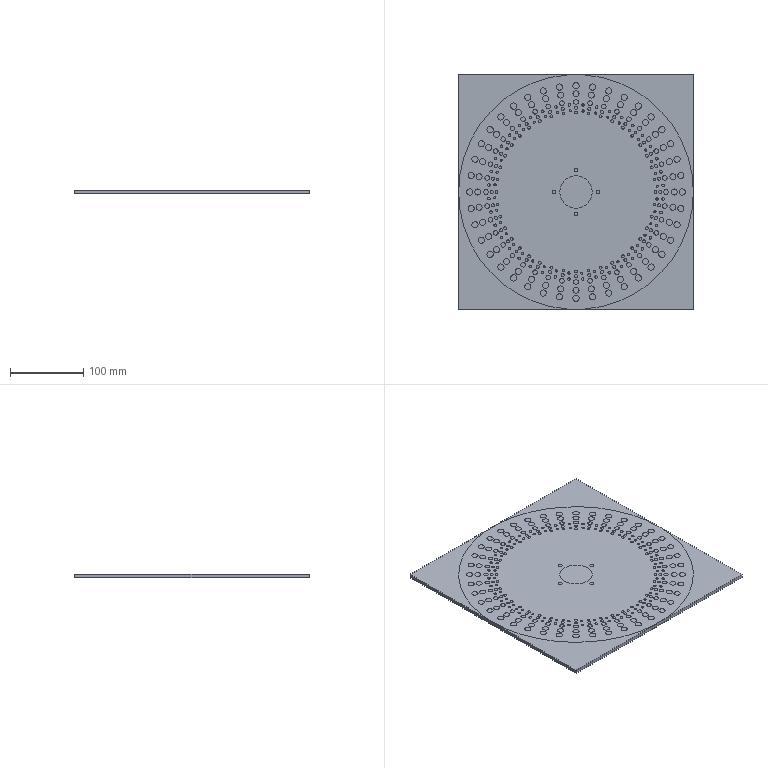NC program | NX | posted with a generic post | part box 320 x 320 x 5 mm
Lines 42718 to 43626 of 63198:
(等高外形_COPY , TOOL : D17R0.8圆鼻飞刀)
N85416 T07 M6
N85418 /M1
N85420 G54
N85422 G17 G0 G90 X-7.068 Y-3.296 S2000 M3
N85424 G43 Z20. H7
N85426 Z0.4
N85428 G94 G1 Z0.2 F1600.
N85430 G3 X-4.906 Y-7.025 R5.1
N85432 X-4.287 Y-7.416 R8.144 F2000.
N85434 X-2.341 Y-8.24 R8.441
N85436 X2.351 Y-8.239 R8.565
N85438 G1 X2.889 Y-8.056
N85440 G3 X4.942 Y-6.996 R7.82
N85442 G1 X5.476 Y-6.59
N85444 X5.768 Y-6.334
N85446 G3 X7.415 Y-4.289 R8.348
N85448 X8.239 Y-2.349 R8.176
N85450 X8.242 Y2.35 R8.507
N85452 G1 X8.238 Y2.355
N85454 G3 X7.418 Y4.288 R8.355
N85456 G1 X7.415 Y4.291
N85458 G3 X5.772 Y6.333 R8.386
N85460 G1 X5.514 Y6.562
N85462 X5.476 Y6.591
N85464 X4.943 Y6.999
N85466 G3 X2.356 Y8.238 R8.466
N85468 G1 X2.352 Y8.242
N85470 G3 X-2.348 Y8.238 R8.563
N85472 X-4.29 Y7.415 R8.305
N85474 X-5.473 Y6.591 R7.498
N85476 X-7.416 Y4.292 R8.562
N85478 X-8.24 Y2.344 R8.479
N85480 X-8.238 Y-2.348 R8.534
N85482 X-5.485 Y-6.578 R8.532
N85484 G1 X-5.47 Y-6.594
N85486 G3 X-4.906 Y-7.025 R8.144
N85488 G1 X-4.6 Y-7.227 Z0.199
N85490 X-4.287 Y-7.416
N85492 X-3.979 Y-7.587 Z0.198
N85494 X-3.665 Y-7.745 Z0.197
N85496 X-3.343 Y-7.887
N85498 X-3.016 Y-8.018 Z0.196
N85500 X-2.682 Y-8.138 Z0.195
N85502 X-2.342 Y-8.24
N85504 X-1.959 Y-8.338 Z0.194
N85506 X-1.571 Y-8.422 Z0.193
N85508 X-1.375 Y-8.455
N85510 X-1.18 Y-8.488 Z0.192
N85512 X-0.983 Y-8.509
N85514 X-0.786 Y-8.531
N85516 X-0.391 Y-8.557 Z0.191
N85518 X0.005 Y-8.568 Z0.19
N85520 X0.203 Y-8.564
N85522 X0.401 Y-8.561
N85524 X0.598 Y-8.546 Z0.189
N85526 X0.796 Y-8.531
N85528 X1.189 Y-8.483 Z0.188
N85530 X1.58 Y-8.42 Z0.187
N85532 X1.968 Y-8.339
N85534 X2.351 Y-8.24 Z0.186
N85536 X2.622 Y-8.155 Z0.185
N85538 X2.893 Y-8.067
N85540 X3.252 Y-7.925 Z0.184
N85542 X3.607 Y-7.77 Z0.183
N85544 X3.954 Y-7.6
N85546 X4.294 Y-7.417 Z0.182
N85548 X4.622 Y-7.213 Z0.181
N85550 X4.942 Y-6.996
N85552 X5.212 Y-6.799 Z0.18
N85554 X5.476 Y-6.59 Z0.179
N85556 X5.623 Y-6.464
N85558 X5.768 Y-6.334
N85560 X6.007 Y-6.107 Z0.178
N85562 X6.239 Y-5.873 Z0.177
N85564 X6.458 Y-5.627
N85566 X6.672 Y-5.376 Z0.176
N85568 X6.873 Y-5.115 Z0.175
N85570 X7.063 Y-4.846
N85572 X7.247 Y-4.572 Z0.174
N85574 X7.416 Y-4.29
N85576 X7.584 Y-3.982 Z0.173
N85578 X7.743 Y-3.669 Z0.172
N85580 X7.885 Y-3.348
N85582 X8.015 Y-3.022 Z0.171
N85584 X8.136 Y-2.688 Z0.17
N85586 X8.24 Y-2.349
N85588 X8.337 Y-1.965 Z0.169
N85590 X8.42 Y-1.577 Z0.168
N85592 X8.486 Y-1.186
N85594 X8.533 Y-0.792 Z0.167
N85596 X8.558 Y-0.396 Z0.166
N85598 X8.575 Y0. Z0.165
N85600 X8.557 Y0.397
N85602 X8.532 Y0.792 Z0.164
N85604 X8.486 Y1.186 Z0.163
N85606 X8.421 Y1.577 Z0.162
N85608 X8.337 Y1.968
N85610 X8.239 Y2.355 Z0.161
N85612 X8.134 Y2.69 Z0.16
N85614 X8.017 Y3.021
N85616 X7.887 Y3.347 Z0.159
N85618 X7.744 Y3.667 Z0.158
N85620 X7.584 Y3.982
N85622 X7.415 Y4.292 Z0.157
N85624 X7.246 Y4.574 Z0.156
N85626 X7.063 Y4.847
N85628 X6.873 Y5.116 Z0.155
N85630 X6.672 Y5.376
N85632 X6.459 Y5.626 Z0.154
N85634 X6.24 Y5.872 Z0.153
N85636 X6.009 Y6.106
N85638 X5.766 Y6.336 Z0.152
N85640 X5.64 Y6.449
N85642 X5.512 Y6.561 Z0.151
N85644 X5.475 Y6.59
N85646 X5.213 Y6.799
N85648 X4.943 Y6.997 Z0.15
N85650 X4.644 Y7.199 Z0.149
N85652 X4.338 Y7.389
N85654 X4.022 Y7.562 Z0.148
N85656 X3.701 Y7.726 Z0.147
N85658 X3.538 Y7.802
N85660 X3.374 Y7.878
N85662 X3.207 Y7.944 Z0.146
N85664 X3.039 Y8.01
N85666 X2.7 Y8.129 Z0.145
N85668 X2.356 Y8.239
N85670 X1.972 Y8.337 Z0.144
N85672 X1.579 Y8.419 Z0.143
N85674 X1.189 Y8.484
N85676 X0.795 Y8.53 Z0.142
N85678 X0.598 Y8.545 Z0.141
N85680 X0.4 Y8.56
N85682 X0.202 Y8.563
N85684 X0.004 Y8.566 Z0.14
N85686 X-0.392 Y8.556
N85688 X-0.787 Y8.531 Z0.139
N85690 X-1.181 Y8.486 Z0.138
N85692 X-1.572 Y8.423 Z0.137
N85694 X-1.962 Y8.338
N85696 X-2.348 Y8.239 Z0.136
N85698 X-2.685 Y8.137 Z0.135
N85700 X-3.017 Y8.018
N85702 X-3.343 Y7.886 Z0.134
N85704 X-3.665 Y7.744 Z0.133
N85706 X-3.981 Y7.586
N85708 X-4.29 Y7.415 Z0.132
N85710 X-4.599 Y7.228 Z0.131
N85712 X-4.899 Y7.029
N85714 X-5.189 Y6.815 Z0.13
N85716 X-5.471 Y6.592 Z0.129
N85718 X-5.759 Y6.345
N85720 X-6.033 Y6.083 Z0.128
N85722 X-6.295 Y5.81 Z0.127
N85724 X-6.545 Y5.526 Z0.126
N85726 X-6.665 Y5.38
N85728 X-6.785 Y5.234
N85730 X-6.896 Y5.081 Z0.125
N85732 X-7.008 Y4.928
N85734 X-7.218 Y4.614 Z0.124
N85736 X-7.415 Y4.291
N85738 X-7.586 Y3.983 Z0.123
N85740 X-7.741 Y3.667 Z0.122
N85742 X-7.886 Y3.345
N85744 X-8.02 Y3.019 Z0.121
N85746 X-8.135 Y2.686 Z0.12
N85748 X-8.239 Y2.349
N85750 X-8.34 Y1.964 Z0.119
N85752 X-8.422 Y1.574 Z0.118
N85754 X-8.484 Y1.184
N85756 X-8.53 Y0.791 Z0.117
N85758 X-8.558 Y0.396 Z0.116
N85760 X-8.57 Y0.001 Z0.115
N85762 X-8.558 Y-0.394
N85764 X-8.53 Y-0.788 Z0.114
N85766 X-8.484 Y-1.181 Z0.113
N85768 X-8.424 Y-1.572 Z0.112
N85770 X-8.341 Y-1.96
N85772 X-8.24 Y-2.342 Z0.111
N85774 X-8.132 Y-2.695 Z0.11
N85776 X-8.01 Y-3.043
N85778 X-7.871 Y-3.382 Z0.109
N85780 X-7.718 Y-3.714 Z0.108
N85782 X-7.553 Y-4.041 Z0.107
N85784 X-7.376 Y-4.361
N85786 X-7.18 Y-4.67 Z0.106
N85788 X-6.975 Y-4.974 Z0.105
N85790 X-6.758 Y-5.268
N85792 X-6.525 Y-5.55 Z0.104
N85794 X-6.282 Y-5.824 Z0.103
N85796 X-6.028 Y-6.088
N85798 X-5.756 Y-6.347 Z0.102
N85800 X-5.471 Y-6.593 Z0.101
N85802 X-5.192 Y-6.813
N85804 X-4.906 Y-7.025 Z0.1
N85806 X-4.6 Y-7.227 Z0.099
N85808 X-4.287 Y-7.416
N85810 X-3.979 Y-7.587 Z0.098
N85812 X-3.665 Y-7.745 Z0.097
N85814 X-3.343 Y-7.887
N85816 X-3.016 Y-8.018 Z0.096
N85818 X-2.682 Y-8.138 Z0.095
N85820 X-2.342 Y-8.24
N85822 X-1.959 Y-8.338 Z0.094
N85824 X-1.571 Y-8.422 Z0.093
N85826 X-1.375 Y-8.455
N85828 X-1.18 Y-8.488 Z0.092
N85830 X-0.983 Y-8.509
N85832 X-0.786 Y-8.531
N85834 X-0.391 Y-8.557 Z0.091
N85836 X0.005 Y-8.568 Z0.09
N85838 X0.203 Y-8.564
N85840 X0.401 Y-8.561
N85842 X0.598 Y-8.546 Z0.089
N85844 X0.796 Y-8.531
N85846 X1.189 Y-8.483 Z0.088
N85848 X1.58 Y-8.42 Z0.087
N85850 X1.968 Y-8.339
N85852 X2.351 Y-8.24 Z0.086
N85854 X2.622 Y-8.155 Z0.085
N85856 X2.893 Y-8.067
N85858 X3.252 Y-7.925 Z0.084
N85860 X3.607 Y-7.77 Z0.083
N85862 X3.954 Y-7.6
N85864 X4.294 Y-7.417 Z0.082
N85866 X4.622 Y-7.213 Z0.081
N85868 X4.942 Y-6.996
N85870 X5.212 Y-6.799 Z0.08
N85872 X5.476 Y-6.59 Z0.079
N85874 X5.623 Y-6.464
N85876 X5.768 Y-6.334
N85878 X6.007 Y-6.107 Z0.078
N85880 X6.239 Y-5.873 Z0.077
N85882 X6.458 Y-5.627
N85884 X6.672 Y-5.376 Z0.076
N85886 X6.873 Y-5.115 Z0.075
N85888 X7.063 Y-4.846
N85890 X7.247 Y-4.572 Z0.074
N85892 X7.416 Y-4.29
N85894 X7.584 Y-3.982 Z0.073
N85896 X7.743 Y-3.669 Z0.072
N85898 X7.885 Y-3.348
N85900 X8.015 Y-3.022 Z0.071
N85902 X8.136 Y-2.688 Z0.07
N85904 X8.24 Y-2.349
N85906 X8.337 Y-1.965 Z0.069
N85908 X8.42 Y-1.577 Z0.068
N85910 X8.486 Y-1.186
N85912 X8.533 Y-0.792 Z0.067
N85914 X8.558 Y-0.396 Z0.066
N85916 X8.575 Y0. Z0.065
N85918 X8.557 Y0.397
N85920 X8.532 Y0.792 Z0.064
N85922 X8.486 Y1.186 Z0.063
N85924 X8.421 Y1.577 Z0.062
N85926 X8.337 Y1.968
N85928 X8.239 Y2.355 Z0.061
N85930 X8.134 Y2.69 Z0.06
N85932 X8.017 Y3.021
N85934 X7.887 Y3.347 Z0.059
N85936 X7.744 Y3.667 Z0.058
N85938 X7.584 Y3.982
N85940 X7.415 Y4.292 Z0.057
N85942 X7.246 Y4.574 Z0.056
N85944 X7.063 Y4.847
N85946 X6.873 Y5.116 Z0.055
N85948 X6.672 Y5.376
N85950 X6.459 Y5.626 Z0.054
N85952 X6.24 Y5.872 Z0.053
N85954 X6.009 Y6.106
N85956 X5.766 Y6.336 Z0.052
N85958 X5.64 Y6.449
N85960 X5.512 Y6.561 Z0.051
N85962 X5.475 Y6.59
N85964 X5.213 Y6.799
N85966 X4.943 Y6.997 Z0.05
N85968 X4.644 Y7.199 Z0.049
N85970 X4.338 Y7.389
N85972 X4.022 Y7.562 Z0.048
N85974 X3.701 Y7.726 Z0.047
N85976 X3.538 Y7.802
N85978 X3.374 Y7.878
N85980 X3.207 Y7.944 Z0.046
N85982 X3.039 Y8.01
N85984 X2.7 Y8.129 Z0.045
N85986 X2.356 Y8.239
N85988 X1.972 Y8.337 Z0.044
N85990 X1.579 Y8.419 Z0.043
N85992 X1.189 Y8.484
N85994 X0.795 Y8.53 Z0.042
N85996 X0.598 Y8.545 Z0.041
N85998 X0.4 Y8.56
N86000 X0.202 Y8.563
N86002 X0.004 Y8.566 Z0.04
N86004 X-0.392 Y8.556
N86006 X-0.787 Y8.531 Z0.039
N86008 X-1.181 Y8.486 Z0.038
N86010 X-1.572 Y8.423 Z0.037
N86012 X-1.962 Y8.338
N86014 X-2.348 Y8.239 Z0.036
N86016 X-2.685 Y8.137 Z0.035
N86018 X-3.017 Y8.018
N86020 X-3.343 Y7.886 Z0.034
N86022 X-3.665 Y7.744 Z0.033
N86024 X-3.981 Y7.586
N86026 X-4.29 Y7.415 Z0.032
N86028 X-4.599 Y7.228 Z0.031
N86030 X-4.899 Y7.029
N86032 X-5.188 Y6.815 Z0.03
N86034 X-5.471 Y6.592 Z0.029
N86036 X-5.759 Y6.345
N86038 X-6.033 Y6.083 Z0.028
N86040 X-6.295 Y5.81 Z0.027
N86042 X-6.545 Y5.526 Z0.026
N86044 X-6.665 Y5.38
N86046 X-6.785 Y5.234
N86048 X-6.896 Y5.081 Z0.025
N86050 X-7.008 Y4.928
N86052 X-7.218 Y4.614 Z0.024
N86054 X-7.415 Y4.291
N86056 X-7.586 Y3.983 Z0.023
N86058 X-7.741 Y3.667 Z0.022
N86060 X-7.886 Y3.345
N86062 X-8.02 Y3.019 Z0.021
N86064 X-8.134 Y2.686 Z0.02
N86066 X-8.239 Y2.349
N86068 X-8.34 Y1.964 Z0.019
N86070 X-8.422 Y1.574 Z0.018
N86072 X-8.484 Y1.184
N86074 X-8.53 Y0.791 Z0.017
N86076 X-8.558 Y0.396 Z0.016
N86078 X-8.57 Y0.001 Z0.015
N86080 X-8.558 Y-0.394
N86082 X-8.53 Y-0.788 Z0.014
N86084 X-8.484 Y-1.181 Z0.013
N86086 X-8.424 Y-1.572 Z0.012
N86088 X-8.341 Y-1.96
N86090 X-8.24 Y-2.342 Z0.011
N86092 X-8.132 Y-2.695 Z0.01
N86094 X-8.01 Y-3.043
N86096 X-7.871 Y-3.382 Z0.009
N86098 X-7.718 Y-3.714 Z0.008
N86100 X-7.553 Y-4.041 Z0.007
N86102 X-7.376 Y-4.361
N86104 X-7.18 Y-4.67 Z0.006
N86106 X-6.975 Y-4.974 Z0.005
N86108 X-6.758 Y-5.268
N86110 X-6.525 Y-5.55 Z0.004
N86112 X-6.282 Y-5.824 Z0.003
N86114 X-6.028 Y-6.088
N86116 X-5.756 Y-6.347 Z0.002
N86118 X-5.471 Y-6.593 Z0.001
N86120 X-5.192 Y-6.813
N86122 X-4.906 Y-7.025 Z0.
N86124 X-4.6 Y-7.227 Z-0.001
N86126 X-4.287 Y-7.416
N86128 X-3.979 Y-7.587 Z-0.002
N86130 X-3.665 Y-7.745 Z-0.003
N86132 X-3.343 Y-7.887
N86134 X-3.016 Y-8.018 Z-0.004
N86136 X-2.682 Y-8.138 Z-0.005
N86138 X-2.342 Y-8.24
N86140 X-1.959 Y-8.338 Z-0.006
N86142 X-1.571 Y-8.422 Z-0.007
N86144 X-1.375 Y-8.455
N86146 X-1.18 Y-8.488 Z-0.008
N86148 X-0.983 Y-8.509
N86150 X-0.786 Y-8.531
N86152 X-0.391 Y-8.557 Z-0.009
N86154 X0.005 Y-8.568 Z-0.01
N86156 X0.203 Y-8.564
N86158 X0.401 Y-8.561
N86160 X0.598 Y-8.546 Z-0.011
N86162 X0.796 Y-8.531
N86164 X1.189 Y-8.483 Z-0.012
N86166 X1.58 Y-8.42 Z-0.013
N86168 X1.968 Y-8.339
N86170 X2.351 Y-8.24 Z-0.014
N86172 X2.622 Y-8.155 Z-0.015
N86174 X2.893 Y-8.067
N86176 X3.252 Y-7.925 Z-0.016
N86178 X3.607 Y-7.77 Z-0.017
N86180 X3.954 Y-7.6
N86182 X4.294 Y-7.417 Z-0.018
N86184 X4.622 Y-7.213 Z-0.019
N86186 X4.942 Y-6.996
N86188 X5.212 Y-6.799 Z-0.02
N86190 X5.476 Y-6.59 Z-0.021
N86192 X5.623 Y-6.464
N86194 X5.768 Y-6.334
N86196 X6.007 Y-6.107 Z-0.022
N86198 X6.239 Y-5.873 Z-0.023
N86200 X6.458 Y-5.627
N86202 X6.672 Y-5.376 Z-0.024
N86204 X6.873 Y-5.115 Z-0.025
N86206 X7.063 Y-4.846
N86208 X7.247 Y-4.572 Z-0.026
N86210 X7.416 Y-4.29
N86212 X7.584 Y-3.982 Z-0.027
N86214 X7.743 Y-3.669 Z-0.028
N86216 X7.885 Y-3.348
N86218 X8.015 Y-3.022 Z-0.029
N86220 X8.136 Y-2.688 Z-0.03
N86222 X8.24 Y-2.349
N86224 X8.337 Y-1.965 Z-0.031
N86226 X8.42 Y-1.577 Z-0.032
N86228 X8.486 Y-1.186
N86230 X8.533 Y-0.792 Z-0.033
N86232 X8.558 Y-0.396 Z-0.034
N86234 X8.575 Y0. Z-0.035
N86236 X8.557 Y0.397
N86238 X8.532 Y0.792 Z-0.036
N86240 X8.486 Y1.186 Z-0.037
N86242 X8.421 Y1.577 Z-0.038
N86244 X8.337 Y1.968
N86246 X8.239 Y2.355 Z-0.039
N86248 X8.134 Y2.69 Z-0.04
N86250 X8.017 Y3.021
N86252 X7.887 Y3.347 Z-0.041
N86254 X7.744 Y3.667 Z-0.042
N86256 X7.584 Y3.982
N86258 X7.415 Y4.292 Z-0.043
N86260 X7.246 Y4.574 Z-0.044
N86262 X7.063 Y4.847
N86264 X6.873 Y5.116 Z-0.045
N86266 X6.672 Y5.376
N86268 X6.459 Y5.626 Z-0.046
N86270 X6.24 Y5.872 Z-0.047
N86272 X6.009 Y6.106
N86274 X5.766 Y6.336 Z-0.048
N86276 X5.64 Y6.449
N86278 X5.512 Y6.561 Z-0.049
N86280 X5.475 Y6.59
N86282 X5.213 Y6.799
N86284 X4.943 Y6.997 Z-0.05
N86286 X4.644 Y7.199 Z-0.051
N86288 X4.338 Y7.389
N86290 X4.022 Y7.562 Z-0.052
N86292 X3.701 Y7.726 Z-0.053
N86294 X3.538 Y7.802
N86296 X3.374 Y7.878
N86298 X3.207 Y7.944 Z-0.054
N86300 X3.039 Y8.01
N86302 X2.7 Y8.129 Z-0.055
N86304 X2.356 Y8.239
N86306 X1.972 Y8.337 Z-0.056
N86308 X1.579 Y8.419 Z-0.057
N86310 X1.189 Y8.484
N86312 X0.795 Y8.53 Z-0.058
N86314 X0.598 Y8.545 Z-0.059
N86316 X0.4 Y8.56
N86318 X0.202 Y8.563
N86320 X0.004 Y8.566 Z-0.06
N86322 X-0.392 Y8.556
N86324 X-0.787 Y8.531 Z-0.061
N86326 X-1.181 Y8.486 Z-0.062
N86328 X-1.572 Y8.423 Z-0.063
N86330 X-1.962 Y8.338
N86332 X-2.348 Y8.239 Z-0.064
N86334 X-2.685 Y8.137 Z-0.065
N86336 X-3.017 Y8.018
N86338 X-3.343 Y7.886 Z-0.066
N86340 X-3.665 Y7.744 Z-0.067
N86342 X-3.981 Y7.586
N86344 X-4.29 Y7.415 Z-0.068
N86346 X-4.599 Y7.228 Z-0.069
N86348 X-4.899 Y7.029
N86350 X-5.188 Y6.815 Z-0.07
N86352 X-5.471 Y6.592 Z-0.071
N86354 X-5.759 Y6.345
N86356 X-6.033 Y6.083 Z-0.072
N86358 X-6.295 Y5.81 Z-0.073
N86360 X-6.545 Y5.526 Z-0.074
N86362 X-6.665 Y5.38
N86364 X-6.785 Y5.234
N86366 X-6.896 Y5.081 Z-0.075
N86368 X-7.008 Y4.928
N86370 X-7.218 Y4.614 Z-0.076
N86372 X-7.415 Y4.291
N86374 X-7.586 Y3.983 Z-0.077
N86376 X-7.741 Y3.667 Z-0.078
N86378 X-7.886 Y3.345
N86380 X-8.02 Y3.019 Z-0.079
N86382 X-8.134 Y2.686 Z-0.08
N86384 X-8.239 Y2.349
N86386 X-8.34 Y1.964 Z-0.081
N86388 X-8.422 Y1.574 Z-0.082
N86390 X-8.484 Y1.184
N86392 X-8.53 Y0.791 Z-0.083
N86394 X-8.558 Y0.396 Z-0.084
N86396 X-8.57 Y0.001 Z-0.085
N86398 X-8.558 Y-0.394
N86400 X-8.53 Y-0.788 Z-0.086
N86402 X-8.484 Y-1.181 Z-0.087
N86404 X-8.424 Y-1.572 Z-0.088
N86406 X-8.341 Y-1.96
N86408 X-8.24 Y-2.342 Z-0.089
N86410 X-8.132 Y-2.695 Z-0.09
N86412 X-8.01 Y-3.043
N86414 X-7.871 Y-3.382 Z-0.091
N86416 X-7.718 Y-3.714 Z-0.092
N86418 X-7.553 Y-4.041 Z-0.093
N86420 X-7.376 Y-4.361
N86422 X-7.18 Y-4.67 Z-0.094
N86424 X-6.975 Y-4.974 Z-0.095
N86426 X-6.757 Y-5.268
N86428 X-6.525 Y-5.55 Z-0.096
N86430 X-6.282 Y-5.824 Z-0.097
N86432 X-6.028 Y-6.088
N86434 X-5.756 Y-6.347 Z-0.098
N86436 X-5.471 Y-6.593 Z-0.099
N86438 X-5.192 Y-6.813
N86440 X-4.906 Y-7.025 Z-0.1
N86442 X-4.6 Y-7.227 Z-0.101
N86444 X-4.287 Y-7.416
N86446 X-3.979 Y-7.587 Z-0.102
N86448 X-3.665 Y-7.745 Z-0.103
N86450 X-3.343 Y-7.887
N86452 X-3.016 Y-8.018 Z-0.104
N86454 X-2.682 Y-8.138 Z-0.105
N86456 X-2.342 Y-8.24
N86458 X-1.959 Y-8.338 Z-0.106
N86460 X-1.571 Y-8.422 Z-0.107
N86462 X-1.375 Y-8.455
N86464 X-1.18 Y-8.488 Z-0.108
N86466 X-0.983 Y-8.509
N86468 X-0.786 Y-8.531
N86470 X-0.391 Y-8.557 Z-0.109
N86472 X0.005 Y-8.568 Z-0.11
N86474 X0.203 Y-8.564
N86476 X0.401 Y-8.561
N86478 X0.598 Y-8.546 Z-0.111
N86480 X0.796 Y-8.531
N86482 X1.189 Y-8.483 Z-0.112
N86484 X1.58 Y-8.42 Z-0.113
N86486 X1.968 Y-8.339
N86488 X2.351 Y-8.24 Z-0.114
N86490 X2.622 Y-8.155 Z-0.115
N86492 X2.893 Y-8.067
N86494 X3.252 Y-7.925 Z-0.116
N86496 X3.607 Y-7.77 Z-0.117
N86498 X3.954 Y-7.6
N86500 X4.294 Y-7.417 Z-0.118
N86502 X4.622 Y-7.213 Z-0.119
N86504 X4.942 Y-6.996
N86506 X5.212 Y-6.799 Z-0.12
N86508 X5.476 Y-6.59 Z-0.121
N86510 X5.623 Y-6.464
N86512 X5.768 Y-6.334
N86514 X6.007 Y-6.107 Z-0.122
N86516 X6.239 Y-5.873 Z-0.123
N86518 X6.458 Y-5.627
N86520 X6.672 Y-5.376 Z-0.124
N86522 X6.873 Y-5.115 Z-0.125
N86524 X7.063 Y-4.846
N86526 X7.247 Y-4.572 Z-0.126
N86528 X7.416 Y-4.29
N86530 X7.584 Y-3.982 Z-0.127
N86532 X7.743 Y-3.669 Z-0.128
N86534 X7.885 Y-3.348
N86536 X8.015 Y-3.022 Z-0.129
N86538 X8.136 Y-2.688 Z-0.13
N86540 X8.24 Y-2.349
N86542 X8.337 Y-1.965 Z-0.131
N86544 X8.42 Y-1.577 Z-0.132
N86546 X8.486 Y-1.186
N86548 X8.533 Y-0.792 Z-0.133
N86550 X8.558 Y-0.396 Z-0.134
N86552 X8.575 Y0. Z-0.135
N86554 X8.557 Y0.397
N86556 X8.532 Y0.792 Z-0.136
N86558 X8.486 Y1.186 Z-0.137
N86560 X8.421 Y1.577 Z-0.138
N86562 X8.337 Y1.968
N86564 X8.239 Y2.355 Z-0.139
N86566 X8.134 Y2.69 Z-0.14
N86568 X8.017 Y3.021
N86570 X7.887 Y3.347 Z-0.141
N86572 X7.744 Y3.667 Z-0.142
N86574 X7.584 Y3.982
N86576 X7.415 Y4.292 Z-0.143
N86578 X7.246 Y4.574 Z-0.144
N86580 X7.063 Y4.847
N86582 X6.873 Y5.116 Z-0.145
N86584 X6.672 Y5.376
N86586 X6.459 Y5.626 Z-0.146
N86588 X6.24 Y5.872 Z-0.147
N86590 X6.009 Y6.106
N86592 X5.766 Y6.336 Z-0.148
N86594 X5.64 Y6.449
N86596 X5.512 Y6.561 Z-0.149
N86598 X5.475 Y6.59
N86600 X5.213 Y6.799
N86602 X4.943 Y6.997 Z-0.15
N86604 X4.644 Y7.199 Z-0.151
N86606 X4.338 Y7.389
N86608 X4.022 Y7.562 Z-0.152
N86610 X3.701 Y7.726 Z-0.153
N86612 X3.538 Y7.802
N86614 X3.374 Y7.878
N86616 X3.207 Y7.944 Z-0.154
N86618 X3.039 Y8.01
N86620 X2.7 Y8.129 Z-0.155
N86622 X2.356 Y8.239
N86624 X1.972 Y8.337 Z-0.156
N86626 X1.579 Y8.419 Z-0.157
N86628 X1.189 Y8.484
N86630 X0.795 Y8.53 Z-0.158
N86632 X0.598 Y8.545 Z-0.159
N86634 X0.4 Y8.56
N86636 X0.202 Y8.565
N86638 X0.004 Y8.566 Z-0.16
N86640 X-0.392 Y8.556
N86642 X-0.787 Y8.531 Z-0.161
N86644 X-1.181 Y8.486 Z-0.162
N86646 X-1.572 Y8.423 Z-0.163
N86648 X-1.962 Y8.338
N86650 X-2.348 Y8.239 Z-0.164
N86652 X-2.685 Y8.137 Z-0.165
N86654 X-3.017 Y8.018
N86656 X-3.343 Y7.886 Z-0.166
N86658 X-3.665 Y7.744 Z-0.167
N86660 X-3.981 Y7.586
N86662 X-4.29 Y7.415 Z-0.168
N86664 X-4.599 Y7.228 Z-0.169
N86666 X-4.899 Y7.029
N86668 X-5.188 Y6.815 Z-0.17
N86670 X-5.471 Y6.592 Z-0.171
N86672 X-5.759 Y6.345
N86674 X-6.033 Y6.083 Z-0.172
N86676 X-6.295 Y5.81 Z-0.173
N86678 X-6.545 Y5.526 Z-0.174
N86680 X-6.665 Y5.38
N86682 X-6.785 Y5.234
N86684 X-6.896 Y5.081 Z-0.175
N86686 X-7.008 Y4.928
N86688 X-7.218 Y4.614 Z-0.176
N86690 X-7.415 Y4.291
N86692 X-7.586 Y3.983 Z-0.177
N86694 X-7.741 Y3.667 Z-0.178
N86696 X-7.886 Y3.345
N86698 X-8.02 Y3.019 Z-0.179
N86700 X-8.134 Y2.686 Z-0.18
N86702 X-8.239 Y2.349
N86704 X-8.34 Y1.964 Z-0.181
N86706 X-8.422 Y1.574 Z-0.182
N86708 X-8.484 Y1.184
N86710 X-8.53 Y0.791 Z-0.183
N86712 X-8.558 Y0.396 Z-0.184
N86714 X-8.57 Y0.001 Z-0.185
N86716 X-8.558 Y-0.394
N86718 X-8.53 Y-0.788 Z-0.186
N86720 X-8.484 Y-1.181 Z-0.187
N86722 X-8.424 Y-1.572 Z-0.188
N86724 X-8.341 Y-1.96
N86726 X-8.24 Y-2.342 Z-0.189
N86728 X-8.132 Y-2.695 Z-0.19
N86730 X-8.01 Y-3.043
N86732 X-7.871 Y-3.382 Z-0.191
N86734 X-7.718 Y-3.714 Z-0.192
N86736 X-7.553 Y-4.041 Z-0.193
N86738 X-7.376 Y-4.361
N86740 X-7.18 Y-4.67 Z-0.194
N86742 X-6.975 Y-4.974 Z-0.195
N86744 X-6.757 Y-5.268
N86746 X-6.525 Y-5.55 Z-0.196
N86748 X-6.282 Y-5.824 Z-0.197
N86750 X-6.028 Y-6.088
N86752 X-5.756 Y-6.347 Z-0.198
N86754 X-5.471 Y-6.593 Z-0.199
N86756 X-5.192 Y-6.813
N86758 X-4.906 Y-7.025 Z-0.2
N86760 X-4.6 Y-7.227 Z-0.201
N86762 X-4.287 Y-7.416
N86764 X-3.979 Y-7.587 Z-0.202
N86766 X-3.665 Y-7.745 Z-0.203
N86768 X-3.343 Y-7.887
N86770 X-3.016 Y-8.018 Z-0.204
N86772 X-2.682 Y-8.138 Z-0.205
N86774 X-2.342 Y-8.24
N86776 X-1.959 Y-8.338 Z-0.206
N86778 X-1.571 Y-8.422 Z-0.207
N86780 X-1.375 Y-8.455
N86782 X-1.18 Y-8.488 Z-0.208
N86784 X-0.983 Y-8.509
N86786 X-0.786 Y-8.531
N86788 X-0.391 Y-8.557 Z-0.209
N86790 X0.005 Y-8.568 Z-0.21
N86792 X0.203 Y-8.564
N86794 X0.401 Y-8.561
N86796 X0.598 Y-8.546 Z-0.211
N86798 X0.796 Y-8.531
N86800 X1.189 Y-8.483 Z-0.212
N86802 X1.58 Y-8.42 Z-0.213
N86804 X1.968 Y-8.339
N86806 X2.351 Y-8.24 Z-0.214
N86808 X2.622 Y-8.155 Z-0.215
N86810 X2.893 Y-8.067
N86812 X3.252 Y-7.925 Z-0.216
N86814 X3.607 Y-7.77 Z-0.217
N86816 X3.954 Y-7.6
N86818 X4.294 Y-7.417 Z-0.218
N86820 X4.622 Y-7.213 Z-0.219
N86822 X4.942 Y-6.996
N86824 X5.212 Y-6.799 Z-0.22
N86826 X5.476 Y-6.59 Z-0.221
N86828 X5.623 Y-6.464
N86830 X5.768 Y-6.334
N86832 X6.007 Y-6.107 Z-0.222
N86834 X6.239 Y-5.873 Z-0.223
N86836 X6.458 Y-5.627
N86838 X6.672 Y-5.376 Z-0.224
N86840 X6.873 Y-5.115 Z-0.225
N86842 X7.063 Y-4.846
N86844 X7.247 Y-4.572 Z-0.226
N86846 X7.416 Y-4.29
N86848 X7.584 Y-3.982 Z-0.227
N86850 X7.743 Y-3.669 Z-0.228
N86852 X7.885 Y-3.348
N86854 X8.015 Y-3.022 Z-0.229
N86856 X8.136 Y-2.688 Z-0.23
N86858 X8.24 Y-2.349
N86860 X8.337 Y-1.965 Z-0.231
N86862 X8.42 Y-1.577 Z-0.232
N86864 X8.486 Y-1.186
N86866 X8.533 Y-0.792 Z-0.233
N86868 X8.558 Y-0.396 Z-0.234
N86870 X8.575 Y0. Z-0.235
N86872 X8.557 Y0.397
N86874 X8.532 Y0.792 Z-0.236
N86876 X8.486 Y1.186 Z-0.237
N86878 X8.421 Y1.577 Z-0.238
N86880 X8.337 Y1.968
N86882 X8.239 Y2.355 Z-0.239
N86884 X8.134 Y2.69 Z-0.24
N86886 X8.017 Y3.021
N86888 X7.887 Y3.347 Z-0.241
N86890 X7.744 Y3.667 Z-0.242
N86892 X7.584 Y3.982
N86894 X7.415 Y4.292 Z-0.243
N86896 X7.246 Y4.574 Z-0.244
N86898 X7.063 Y4.847
N86900 X6.873 Y5.116 Z-0.245
N86902 X6.672 Y5.376
N86904 X6.459 Y5.626 Z-0.246
N86906 X6.24 Y5.872 Z-0.247
N86908 X6.009 Y6.106
N86910 X5.765 Y6.336 Z-0.248
N86912 X5.64 Y6.449
N86914 X5.512 Y6.561 Z-0.249
N86916 X5.475 Y6.59
N86918 X5.213 Y6.799
N86920 X4.943 Y6.997 Z-0.25
N86922 X4.644 Y7.199 Z-0.251
N86924 X4.338 Y7.389
N86926 X4.022 Y7.562 Z-0.252
N86928 X3.701 Y7.726 Z-0.253
N86930 X3.374 Y7.878
N86932 X3.039 Y8.01 Z-0.254
N86934 X2.7 Y8.129 Z-0.255
N86936 X2.356 Y8.239
N86938 X1.972 Y8.337 Z-0.256
N86940 X1.579 Y8.419 Z-0.257
N86942 X1.189 Y8.484
N86944 X0.795 Y8.53 Z-0.258
N86946 X0.598 Y8.545 Z-0.259
N86948 X0.4 Y8.56
N86950 X0.202 Y8.565
N86952 X0.004 Y8.566 Z-0.26
N86954 X-0.392 Y8.556
N86956 X-0.787 Y8.531 Z-0.261
N86958 X-1.181 Y8.486 Z-0.262
N86960 X-1.572 Y8.423 Z-0.263
N86962 X-1.962 Y8.338
N86964 X-2.348 Y8.239 Z-0.264
N86966 X-2.685 Y8.137 Z-0.265
N86968 X-3.017 Y8.018
N86970 X-3.343 Y7.886 Z-0.266
N86972 X-3.665 Y7.744 Z-0.267
N86974 X-3.981 Y7.586
N86976 X-4.29 Y7.415 Z-0.268
N86978 X-4.599 Y7.228 Z-0.269
N86980 X-4.899 Y7.029
N86982 X-5.188 Y6.815 Z-0.27
N86984 X-5.471 Y6.592 Z-0.271
N86986 X-5.759 Y6.345
N86988 X-6.033 Y6.083 Z-0.272
N86990 X-6.295 Y5.81 Z-0.273
N86992 X-6.545 Y5.526 Z-0.274
N86994 X-6.665 Y5.38
N86996 X-6.785 Y5.234
N86998 X-6.896 Y5.081 Z-0.275
N87000 X-7.008 Y4.928
N87002 X-7.218 Y4.614 Z-0.276
N87004 X-7.415 Y4.291
N87006 X-7.586 Y3.983 Z-0.277
N87008 X-7.741 Y3.667 Z-0.278
N87010 X-7.886 Y3.345
N87012 X-8.02 Y3.019 Z-0.279
N87014 X-8.134 Y2.686 Z-0.28
N87016 X-8.239 Y2.349
N87018 X-8.34 Y1.964 Z-0.281
N87020 X-8.422 Y1.574 Z-0.282
N87022 X-8.484 Y1.184
N87024 X-8.53 Y0.791 Z-0.283
N87026 X-8.558 Y0.396 Z-0.284
N87028 X-8.57 Y0.001 Z-0.285
N87030 X-8.558 Y-0.394
N87032 X-8.53 Y-0.788 Z-0.286
N87034 X-8.484 Y-1.181 Z-0.287
N87036 X-8.424 Y-1.572 Z-0.288
N87038 X-8.341 Y-1.96
N87040 X-8.24 Y-2.342 Z-0.289
N87042 X-8.132 Y-2.695 Z-0.29
N87044 X-8.01 Y-3.043
N87046 X-7.871 Y-3.382 Z-0.291
N87048 X-7.718 Y-3.715 Z-0.292
N87050 X-7.553 Y-4.041 Z-0.293
N87052 X-7.376 Y-4.361
N87054 X-7.18 Y-4.67 Z-0.294
N87056 X-6.975 Y-4.974 Z-0.295
N87058 X-6.757 Y-5.268
N87060 X-6.525 Y-5.55 Z-0.296
N87062 X-6.282 Y-5.824 Z-0.297
N87064 X-6.028 Y-6.088
N87066 X-5.756 Y-6.347 Z-0.298
N87068 X-5.471 Y-6.593 Z-0.299
N87070 X-5.192 Y-6.813
N87072 X-4.906 Y-7.025 Z-0.3
N87074 X-4.6 Y-7.227 Z-0.301
N87076 X-4.287 Y-7.416
N87078 X-3.979 Y-7.587 Z-0.302
N87080 X-3.665 Y-7.745 Z-0.303
N87082 X-3.343 Y-7.887
N87084 X-3.016 Y-8.018 Z-0.304
N87086 X-2.682 Y-8.138 Z-0.305
N87088 X-2.342 Y-8.24
N87090 X-1.959 Y-8.338 Z-0.306
N87092 X-1.571 Y-8.422 Z-0.307
N87094 X-1.375 Y-8.455
N87096 X-1.18 Y-8.488 Z-0.308
N87098 X-0.983 Y-8.509
N87100 X-0.786 Y-8.531
N87102 X-0.391 Y-8.557 Z-0.309
N87104 X0.005 Y-8.568 Z-0.31
N87106 X0.203 Y-8.564
N87108 X0.401 Y-8.561
N87110 X0.598 Y-8.546 Z-0.311
N87112 X0.796 Y-8.531
N87114 X1.189 Y-8.483 Z-0.312
N87116 X1.58 Y-8.42 Z-0.313
N87118 X1.968 Y-8.339
N87120 X2.351 Y-8.24 Z-0.314
N87122 X2.622 Y-8.155 Z-0.315
N87124 X2.893 Y-8.067
N87126 X3.252 Y-7.925 Z-0.316
N87128 X3.607 Y-7.77 Z-0.317
N87130 X3.954 Y-7.6
N87132 X4.294 Y-7.417 Z-0.318
N87134 X4.622 Y-7.213 Z-0.319
N87136 X4.942 Y-6.996
N87138 X5.212 Y-6.799 Z-0.32
N87140 X5.476 Y-6.59 Z-0.321
N87142 X5.623 Y-6.464
N87144 X5.768 Y-6.334
N87146 X6.007 Y-6.107 Z-0.322
N87148 X6.239 Y-5.873 Z-0.323
N87150 X6.458 Y-5.627
N87152 X6.672 Y-5.376 Z-0.324
N87154 X6.873 Y-5.115 Z-0.325
N87156 X7.063 Y-4.846
N87158 X7.247 Y-4.572 Z-0.326
N87160 X7.416 Y-4.29
N87162 X7.584 Y-3.982 Z-0.327
N87164 X7.743 Y-3.669 Z-0.328
N87166 X7.885 Y-3.348
N87168 X8.015 Y-3.022 Z-0.329
N87170 X8.136 Y-2.688 Z-0.33
N87172 X8.24 Y-2.349
N87174 X8.337 Y-1.965 Z-0.331
N87176 X8.42 Y-1.577 Z-0.332
N87178 X8.486 Y-1.186
N87180 X8.533 Y-0.792 Z-0.333
N87182 X8.558 Y-0.396 Z-0.334
N87184 X8.575 Y0. Z-0.335
N87186 X8.557 Y0.397
N87188 X8.532 Y0.792 Z-0.336
N87190 X8.486 Y1.186 Z-0.337
N87192 X8.421 Y1.577 Z-0.338
N87194 X8.337 Y1.968
N87196 X8.239 Y2.355 Z-0.339
N87198 X8.134 Y2.69 Z-0.34
N87200 X8.017 Y3.021
N87202 X7.887 Y3.347 Z-0.341
N87204 X7.744 Y3.667 Z-0.342
N87206 X7.584 Y3.982
N87208 X7.415 Y4.292 Z-0.343
N87210 X7.246 Y4.574 Z-0.344
N87212 X7.063 Y4.847
N87214 X6.873 Y5.116 Z-0.345
N87216 X6.672 Y5.376
N87218 X6.459 Y5.626 Z-0.346
N87220 X6.24 Y5.872 Z-0.347
N87222 X6.009 Y6.106
N87224 X5.765 Y6.336 Z-0.348
N87226 X5.64 Y6.449